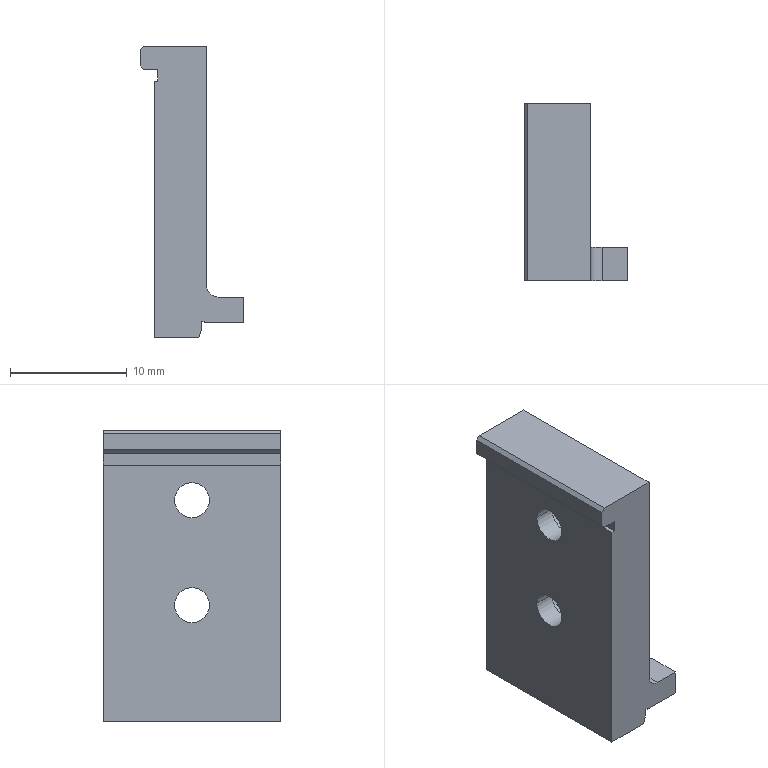Part | NX | 1 solid | 31 faces | box 8.9 x 15.2 x 25 mm | volume 1620 mm3 | plane 22 | cylinder 9 | commonest cylinder face diameters 3 x4 5 x4 2 x1
STEP:
#1=CARTESIAN_POINT('',(-1.77,0.,-1.43));
#2=VERTEX_POINT('',#1);
#3=CARTESIAN_POINT('',(-2.025,0.,-2.13));
#4=VERTEX_POINT('',#3);
#5=CARTESIAN_POINT('',(-1.25,0.,0.));
#6=DIRECTION('',(-0.342,0.,-0.9397));
#7=VECTOR('',#6,1000.);
#8=LINE('',#5,#7);
#9=EDGE_CURVE('',#2,#4,#8,.T.);
#10=ORIENTED_EDGE('',*,*,#9,.T.);
#11=CARTESIAN_POINT('',(-5.85,0.,-2.13));
#12=VERTEX_POINT('',#11);
#13=CARTESIAN_POINT('',(0.,0.,-2.13));
#14=DIRECTION('',(1.,0.,0.));
#15=VECTOR('',#14,1000.);
#16=LINE('',#13,#15);
#17=EDGE_CURVE('',#12,#4,#16,.T.);
#18=ORIENTED_EDGE('',*,*,#17,.F.);
#19=CARTESIAN_POINT('',(-5.85,0.,19.87));
#20=VERTEX_POINT('',#19);
#21=CARTESIAN_POINT('',(-5.85,0.,0.));
#22=DIRECTION('',(0.,0.,1.));
#23=VECTOR('',#22,1000.);
#24=LINE('',#21,#23);
#25=EDGE_CURVE('',#12,#20,#24,.T.);
#26=ORIENTED_EDGE('',*,*,#25,.T.);
#27=CARTESIAN_POINT('',(-5.55,0.,19.87));
#28=VERTEX_POINT('',#27);
#29=CARTESIAN_POINT('',(0.,0.,19.87));
#30=DIRECTION('',(1.,0.,0.));
#31=VECTOR('',#30,1000.);
#32=LINE('',#29,#31);
#33=EDGE_CURVE('',#20,#28,#32,.T.);
#34=ORIENTED_EDGE('',*,*,#33,.T.);
#35=CARTESIAN_POINT('',(-5.55,0.,20.87));
#36=VERTEX_POINT('',#35);
#37=CARTESIAN_POINT('',(-5.55,0.,0.));
#38=DIRECTION('',(0.,0.,1.));
#39=VECTOR('',#38,1000.);
#40=LINE('',#37,#39);
#41=EDGE_CURVE('',#28,#36,#40,.T.);
#42=ORIENTED_EDGE('',*,*,#41,.T.);
#43=CARTESIAN_POINT('',(-6.75,0.,20.87));
#44=VERTEX_POINT('',#43);
#45=CARTESIAN_POINT('',(0.,0.,20.87));
#46=DIRECTION('',(-1.,0.,0.));
#47=VECTOR('',#46,1000.);
#48=LINE('',#45,#47);
#49=EDGE_CURVE('',#36,#44,#48,.T.);
#50=ORIENTED_EDGE('',*,*,#49,.T.);
#51=CARTESIAN_POINT('',(-7.05,0.,21.17));
#52=VERTEX_POINT('',#51);
#53=CARTESIAN_POINT('',(14.12,0.,0.));
#54=DIRECTION('',(0.7071,0.,-0.7071));
#55=VECTOR('',#54,1000.);
#56=LINE('',#53,#55);
#57=EDGE_CURVE('',#52,#44,#56,.T.);
#58=ORIENTED_EDGE('',*,*,#57,.F.);
#59=CARTESIAN_POINT('',(-7.05,0.,22.57));
#60=VERTEX_POINT('',#59);
#61=CARTESIAN_POINT('',(-7.05,0.,0.));
#62=DIRECTION('',(0.,0.,1.));
#63=VECTOR('',#62,1000.);
#64=LINE('',#61,#63);
#65=EDGE_CURVE('',#52,#60,#64,.T.);
#66=ORIENTED_EDGE('',*,*,#65,.T.);
#67=CARTESIAN_POINT('',(-6.75,0.,22.87));
#68=VERTEX_POINT('',#67);
#69=CARTESIAN_POINT('',(-29.62,0.,0.));
#70=DIRECTION('',(0.7071,0.,0.7071));
#71=VECTOR('',#70,1000.);
#72=LINE('',#69,#71);
#73=EDGE_CURVE('',#60,#68,#72,.T.);
#74=ORIENTED_EDGE('',*,*,#73,.T.);
#75=CARTESIAN_POINT('',(-1.35,0.,22.87));
#76=VERTEX_POINT('',#75);
#77=CARTESIAN_POINT('',(0.,0.,22.87));
#78=DIRECTION('',(1.,0.,0.));
#79=VECTOR('',#78,1000.);
#80=LINE('',#77,#79);
#81=EDGE_CURVE('',#68,#76,#80,.T.);
#82=ORIENTED_EDGE('',*,*,#81,.T.);
#83=CARTESIAN_POINT('',(-1.35,0.,-0.83));
#84=VERTEX_POINT('',#83);
#85=CARTESIAN_POINT('',(-1.35,0.,0.));
#86=DIRECTION('',(0.,0.,-1.));
#87=VECTOR('',#86,1000.);
#88=LINE('',#85,#87);
#89=EDGE_CURVE('',#76,#84,#88,.T.);
#90=ORIENTED_EDGE('',*,*,#89,.T.);
#91=CARTESIAN_POINT('',(-1.57,0.,-0.83));
#92=VERTEX_POINT('',#91);
#93=CARTESIAN_POINT('',(0.,0.,-0.83));
#94=DIRECTION('',(1.,0.,0.));
#95=VECTOR('',#94,1000.);
#96=LINE('',#93,#95);
#97=EDGE_CURVE('',#92,#84,#96,.T.);
#98=ORIENTED_EDGE('',*,*,#97,.F.);
#99=CARTESIAN_POINT('',(-1.57,0.,-0.73));
#100=VERTEX_POINT('',#99);
#101=CARTESIAN_POINT('',(-1.57,0.,0.));
#102=DIRECTION('',(0.,0.,-1.));
#103=VECTOR('',#102,1000.);
#104=LINE('',#101,#103);
#105=EDGE_CURVE('',#100,#92,#104,.T.);
#106=ORIENTED_EDGE('',*,*,#105,.F.);
#107=CARTESIAN_POINT('',(-1.77,0.,-0.73));
#108=VERTEX_POINT('',#107);
#109=CARTESIAN_POINT('',(0.,0.,-0.73));
#110=DIRECTION('',(-1.,0.,0.));
#111=VECTOR('',#110,1000.);
#112=LINE('',#109,#111);
#113=EDGE_CURVE('',#100,#108,#112,.T.);
#114=ORIENTED_EDGE('',*,*,#113,.T.);
#115=CARTESIAN_POINT('',(-1.77,0.,0.));
#116=DIRECTION('',(0.,0.,-1.));
#117=VECTOR('',#116,1000.);
#118=LINE('',#115,#117);
#119=EDGE_CURVE('',#108,#2,#118,.T.);
#120=ORIENTED_EDGE('',*,*,#119,.T.);
#121=EDGE_LOOP('',(#10,#18,#26,#34,#42,#50,#58,#66,#74,#82,#90,#98,#106,#114,#120));
#122=FACE_BOUND('',#121,.T.);
#123=CARTESIAN_POINT('',(0.,0.,0.));
#124=DIRECTION('',(0.,-1.,0.));
#125=DIRECTION('',(0.,0.,-1.));
#126=AXIS2_PLACEMENT_3D('',#123,#124,#125);
#127=PLANE('',#126);
#128=ADVANCED_FACE('',(#122),#127,.F.);
#129=CARTESIAN_POINT('',(-1.77,-15.2,-1.43));
#130=VERTEX_POINT('',#129);
#131=CARTESIAN_POINT('',(-1.77,0.,-1.43));
#132=DIRECTION('',(0.,-1.,0.));
#133=VECTOR('',#132,1000.);
#134=LINE('',#131,#133);
#135=EDGE_CURVE('',#2,#130,#134,.T.);
#136=ORIENTED_EDGE('',*,*,#135,.F.);
#137=ORIENTED_EDGE('',*,*,#119,.F.);
#138=CARTESIAN_POINT('',(-1.77,-15.2,-0.73));
#139=VERTEX_POINT('',#138);
#140=CARTESIAN_POINT('',(-1.77,-15.2,-0.73));
#141=DIRECTION('',(0.,1.,0.));
#142=VECTOR('',#141,1000.);
#143=LINE('',#140,#142);
#144=EDGE_CURVE('',#139,#108,#143,.T.);
#145=ORIENTED_EDGE('',*,*,#144,.F.);
#146=CARTESIAN_POINT('',(-1.77,-15.2,0.));
#147=DIRECTION('',(0.,0.,1.));
#148=VECTOR('',#147,1000.);
#149=LINE('',#146,#148);
#150=EDGE_CURVE('',#130,#139,#149,.T.);
#151=ORIENTED_EDGE('',*,*,#150,.F.);
#152=EDGE_LOOP('',(#136,#137,#145,#151));
#153=FACE_BOUND('',#152,.T.);
#154=CARTESIAN_POINT('',(-1.77,0.,-0.93));
#155=DIRECTION('',(1.,0.,0.));
#156=DIRECTION('',(0.,1.,0.));
#157=AXIS2_PLACEMENT_3D('',#154,#155,#156);
#158=PLANE('',#157);
#159=ADVANCED_FACE('',(#153),#158,.T.);
#160=CARTESIAN_POINT('',(-0.35,-15.2,1.37));
#161=VERTEX_POINT('',#160);
#162=CARTESIAN_POINT('',(1.85,-15.2,1.37));
#163=VERTEX_POINT('',#162);
#164=CARTESIAN_POINT('',(0.,-15.2,1.37));
#165=DIRECTION('',(1.,0.,0.));
#166=VECTOR('',#165,1000.);
#167=LINE('',#164,#166);
#168=EDGE_CURVE('',#161,#163,#167,.T.);
#169=ORIENTED_EDGE('',*,*,#168,.F.);
#170=CARTESIAN_POINT('',(-1.35,-15.2,2.37));
#171=VERTEX_POINT('',#170);
#172=CARTESIAN_POINT('',(-0.35,-15.2,2.37));
#173=DIRECTION('',(0.,1.,0.));
#174=DIRECTION('',(-1.,0.,0.));
#175=AXIS2_PLACEMENT_3D('',#172,#173,#174);
#176=CIRCLE('',#175,1.);
#177=EDGE_CURVE('',#161,#171,#176,.T.);
#178=ORIENTED_EDGE('',*,*,#177,.T.);
#179=CARTESIAN_POINT('',(-1.35,-15.2,22.87));
#180=VERTEX_POINT('',#179);
#181=CARTESIAN_POINT('',(-1.35,-15.2,0.));
#182=DIRECTION('',(0.,0.,1.));
#183=VECTOR('',#182,1000.);
#184=LINE('',#181,#183);
#185=EDGE_CURVE('',#171,#180,#184,.T.);
#186=ORIENTED_EDGE('',*,*,#185,.T.);
#187=CARTESIAN_POINT('',(-6.75,-15.2,22.87));
#188=VERTEX_POINT('',#187);
#189=CARTESIAN_POINT('',(0.,-15.2,22.87));
#190=DIRECTION('',(-1.,0.,0.));
#191=VECTOR('',#190,1000.);
#192=LINE('',#189,#191);
#193=EDGE_CURVE('',#180,#188,#192,.T.);
#194=ORIENTED_EDGE('',*,*,#193,.T.);
#195=CARTESIAN_POINT('',(-7.05,-15.2,22.57));
#196=VERTEX_POINT('',#195);
#197=CARTESIAN_POINT('',(-29.62,-15.2,0.));
#198=DIRECTION('',(-0.7071,0.,-0.7071));
#199=VECTOR('',#198,1000.);
#200=LINE('',#197,#199);
#201=EDGE_CURVE('',#188,#196,#200,.T.);
#202=ORIENTED_EDGE('',*,*,#201,.T.);
#203=CARTESIAN_POINT('',(-7.05,-15.2,21.17));
#204=VERTEX_POINT('',#203);
#205=CARTESIAN_POINT('',(-7.05,-15.2,0.));
#206=DIRECTION('',(0.,0.,-1.));
#207=VECTOR('',#206,1000.);
#208=LINE('',#205,#207);
#209=EDGE_CURVE('',#196,#204,#208,.T.);
#210=ORIENTED_EDGE('',*,*,#209,.T.);
#211=CARTESIAN_POINT('',(-6.75,-15.2,20.87));
#212=VERTEX_POINT('',#211);
#213=CARTESIAN_POINT('',(14.12,-15.2,0.));
#214=DIRECTION('',(-0.7071,0.,0.7071));
#215=VECTOR('',#214,1000.);
#216=LINE('',#213,#215);
#217=EDGE_CURVE('',#212,#204,#216,.T.);
#218=ORIENTED_EDGE('',*,*,#217,.F.);
#219=CARTESIAN_POINT('',(-5.55,-15.2,20.87));
#220=VERTEX_POINT('',#219);
#221=CARTESIAN_POINT('',(0.,-15.2,20.87));
#222=DIRECTION('',(1.,0.,0.));
#223=VECTOR('',#222,1000.);
#224=LINE('',#221,#223);
#225=EDGE_CURVE('',#212,#220,#224,.T.);
#226=ORIENTED_EDGE('',*,*,#225,.T.);
#227=CARTESIAN_POINT('',(-5.55,-15.2,19.87));
#228=VERTEX_POINT('',#227);
#229=CARTESIAN_POINT('',(-5.55,-15.2,0.));
#230=DIRECTION('',(0.,0.,-1.));
#231=VECTOR('',#230,1000.);
#232=LINE('',#229,#231);
#233=EDGE_CURVE('',#220,#228,#232,.T.);
#234=ORIENTED_EDGE('',*,*,#233,.T.);
#235=CARTESIAN_POINT('',(-5.85,-15.2,19.87));
#236=VERTEX_POINT('',#235);
#237=CARTESIAN_POINT('',(0.,-15.2,19.87));
#238=DIRECTION('',(-1.,0.,0.));
#239=VECTOR('',#238,1000.);
#240=LINE('',#237,#239);
#241=EDGE_CURVE('',#228,#236,#240,.T.);
#242=ORIENTED_EDGE('',*,*,#241,.T.);
#243=CARTESIAN_POINT('',(-5.85,-15.2,-2.13));
#244=VERTEX_POINT('',#243);
#245=CARTESIAN_POINT('',(-5.85,-15.2,0.));
#246=DIRECTION('',(0.,0.,-1.));
#247=VECTOR('',#246,1000.);
#248=LINE('',#245,#247);
#249=EDGE_CURVE('',#236,#244,#248,.T.);
#250=ORIENTED_EDGE('',*,*,#249,.T.);
#251=CARTESIAN_POINT('',(-2.025,-15.2,-2.13));
#252=VERTEX_POINT('',#251);
#253=CARTESIAN_POINT('',(0.,-15.2,-2.13));
#254=DIRECTION('',(-1.,0.,0.));
#255=VECTOR('',#254,1000.);
#256=LINE('',#253,#255);
#257=EDGE_CURVE('',#252,#244,#256,.T.);
#258=ORIENTED_EDGE('',*,*,#257,.F.);
#259=CARTESIAN_POINT('',(-1.25,-15.2,0.));
#260=DIRECTION('',(0.342,0.,0.9397));
#261=VECTOR('',#260,1000.);
#262=LINE('',#259,#261);
#263=EDGE_CURVE('',#252,#130,#262,.T.);
#264=ORIENTED_EDGE('',*,*,#263,.T.);
#265=ORIENTED_EDGE('',*,*,#150,.T.);
#266=CARTESIAN_POINT('',(-1.57,-15.2,-0.73));
#267=VERTEX_POINT('',#266);
#268=CARTESIAN_POINT('',(0.,-15.2,-0.73));
#269=DIRECTION('',(1.,0.,0.));
#270=VECTOR('',#269,1000.);
#271=LINE('',#268,#270);
#272=EDGE_CURVE('',#139,#267,#271,.T.);
#273=ORIENTED_EDGE('',*,*,#272,.T.);
#274=CARTESIAN_POINT('',(-1.57,-15.2,-0.83));
#275=VERTEX_POINT('',#274);
#276=CARTESIAN_POINT('',(-1.57,-15.2,0.));
#277=DIRECTION('',(0.,0.,1.));
#278=VECTOR('',#277,1000.);
#279=LINE('',#276,#278);
#280=EDGE_CURVE('',#275,#267,#279,.T.);
#281=ORIENTED_EDGE('',*,*,#280,.F.);
#282=CARTESIAN_POINT('',(1.85,-15.2,-0.83));
#283=VERTEX_POINT('',#282);
#284=CARTESIAN_POINT('',(0.,-15.2,-0.83));
#285=DIRECTION('',(1.,0.,0.));
#286=VECTOR('',#285,1000.);
#287=LINE('',#284,#286);
#288=EDGE_CURVE('',#275,#283,#287,.T.);
#289=ORIENTED_EDGE('',*,*,#288,.T.);
#290=CARTESIAN_POINT('',(1.85,-15.2,0.));
#291=DIRECTION('',(0.,0.,1.));
#292=VECTOR('',#291,1000.);
#293=LINE('',#290,#292);
#294=EDGE_CURVE('',#283,#163,#293,.T.);
#295=ORIENTED_EDGE('',*,*,#294,.T.);
#296=EDGE_LOOP('',(#169,#178,#186,#194,#202,#210,#218,#226,#234,#242,#250,#258,#264,#265,#273,#281,#289,#295));
#297=FACE_BOUND('',#296,.T.);
#298=CARTESIAN_POINT('',(-1.35,-15.2,0.));
#299=DIRECTION('',(0.,1.,0.));
#300=DIRECTION('',(1.,0.,0.));
#301=AXIS2_PLACEMENT_3D('',#298,#299,#300);
#302=PLANE('',#301);
#303=ADVANCED_FACE('',(#297),#302,.F.);
#304=CARTESIAN_POINT('',(-4.05,-5.1,7.87));
#305=VERTEX_POINT('',#304);
#306=CARTESIAN_POINT('',(-4.05,-10.1,7.87));
#307=VERTEX_POINT('',#306);
#308=CARTESIAN_POINT('',(-4.05,-7.6,7.87));
#309=DIRECTION('',(1.,0.,0.));
#310=DIRECTION('',(0.,-1.,0.));
#311=AXIS2_PLACEMENT_3D('',#308,#309,#310);
#312=CIRCLE('',#311,2.5);
#313=EDGE_CURVE('',#305,#307,#312,.T.);
#314=ORIENTED_EDGE('',*,*,#313,.T.);
#315=CARTESIAN_POINT('',(-4.05,-7.6,7.87));
#316=DIRECTION('',(1.,0.,0.));
#317=DIRECTION('',(0.,-1.,0.));
#318=AXIS2_PLACEMENT_3D('',#315,#316,#317);
#319=CIRCLE('',#318,2.5);
#320=EDGE_CURVE('',#307,#305,#319,.T.);
#321=ORIENTED_EDGE('',*,*,#320,.T.);
#322=EDGE_LOOP('',(#314,#321));
#323=FACE_BOUND('',#322,.T.);
#324=CARTESIAN_POINT('',(-4.05,-6.1,7.87));
#325=VERTEX_POINT('',#324);
#326=CARTESIAN_POINT('',(-4.05,-9.1,7.87));
#327=VERTEX_POINT('',#326);
#328=CARTESIAN_POINT('',(-4.05,-7.6,7.87));
#329=DIRECTION('',(1.,0.,0.));
#330=DIRECTION('',(0.,-1.,0.));
#331=AXIS2_PLACEMENT_3D('',#328,#329,#330);
#332=CIRCLE('',#331,1.5);
#333=EDGE_CURVE('',#325,#327,#332,.T.);
#334=ORIENTED_EDGE('',*,*,#333,.F.);
#335=CARTESIAN_POINT('',(-4.05,-7.6,7.87));
#336=DIRECTION('',(1.,0.,0.));
#337=DIRECTION('',(0.,-1.,0.));
#338=AXIS2_PLACEMENT_3D('',#335,#336,#337);
#339=CIRCLE('',#338,1.5);
#340=EDGE_CURVE('',#327,#325,#339,.T.);
#341=ORIENTED_EDGE('',*,*,#340,.F.);
#342=EDGE_LOOP('',(#334,#341));
#343=FACE_BOUND('',#342,.T.);
#344=CARTESIAN_POINT('',(-4.05,-7.6,7.87));
#345=DIRECTION('',(-1.,0.,0.));
#346=DIRECTION('',(0.,0.,1.));
#347=AXIS2_PLACEMENT_3D('',#344,#345,#346);
#348=PLANE('',#347);
#349=ADVANCED_FACE('',(#323,#343),#348,.F.);
#350=ORIENTED_EDGE('',*,*,#257,.T.);
#351=CARTESIAN_POINT('',(-5.85,0.,-2.13));
#352=DIRECTION('',(0.,1.,0.));
#353=VECTOR('',#352,1000.);
#354=LINE('',#351,#353);
#355=EDGE_CURVE('',#244,#12,#354,.T.);
#356=ORIENTED_EDGE('',*,*,#355,.T.);
#357=ORIENTED_EDGE('',*,*,#17,.T.);
#358=CARTESIAN_POINT('',(-2.025,0.,-2.13));
#359=DIRECTION('',(0.,-1.,0.));
#360=VECTOR('',#359,1000.);
#361=LINE('',#358,#360);
#362=EDGE_CURVE('',#4,#252,#361,.T.);
#363=ORIENTED_EDGE('',*,*,#362,.T.);
#364=EDGE_LOOP('',(#350,#356,#357,#363));
#365=FACE_BOUND('',#364,.T.);
#366=CARTESIAN_POINT('',(0.,0.,-2.13));
#367=DIRECTION('',(0.,0.,1.));
#368=DIRECTION('',(1.,0.,0.));
#369=AXIS2_PLACEMENT_3D('',#366,#367,#368);
#370=PLANE('',#369);
#371=ADVANCED_FACE('',(#365),#370,.F.);
#372=ORIENTED_EDGE('',*,*,#9,.F.);
#373=ORIENTED_EDGE('',*,*,#135,.T.);
#374=ORIENTED_EDGE('',*,*,#263,.F.);
#375=ORIENTED_EDGE('',*,*,#362,.F.);
#376=EDGE_LOOP('',(#372,#373,#374,#375));
#377=FACE_BOUND('',#376,.T.);
#378=CARTESIAN_POINT('',(-2.025,-15.2,-2.13));
#379=DIRECTION('',(0.9397,0.,-0.342));
#380=DIRECTION('',(0.,-1.,0.));
#381=AXIS2_PLACEMENT_3D('',#378,#379,#380);
#382=PLANE('',#381);
#383=ADVANCED_FACE('',(#377),#382,.T.);
#384=CARTESIAN_POINT('',(-5.85,0.,19.87));
#385=DIRECTION('',(0.,-1.,0.));
#386=VECTOR('',#385,1000.);
#387=LINE('',#384,#386);
#388=EDGE_CURVE('',#20,#236,#387,.T.);
#389=ORIENTED_EDGE('',*,*,#388,.T.);
#390=ORIENTED_EDGE('',*,*,#241,.F.);
#391=CARTESIAN_POINT('',(-5.55,0.,19.87));
#392=DIRECTION('',(0.,-1.,0.));
#393=VECTOR('',#392,1000.);
#394=LINE('',#391,#393);
#395=EDGE_CURVE('',#28,#228,#394,.T.);
#396=ORIENTED_EDGE('',*,*,#395,.F.);
#397=ORIENTED_EDGE('',*,*,#33,.F.);
#398=EDGE_LOOP('',(#389,#390,#396,#397));
#399=FACE_BOUND('',#398,.T.);
#400=CARTESIAN_POINT('',(-4.85,0.,19.87));
#401=DIRECTION('',(0.,0.,1.));
#402=DIRECTION('',(1.,0.,0.));
#403=AXIS2_PLACEMENT_3D('',#400,#401,#402);
#404=PLANE('',#403);
#405=ADVANCED_FACE('',(#399),#404,.T.);
#406=ORIENTED_EDGE('',*,*,#395,.T.);
#407=ORIENTED_EDGE('',*,*,#233,.F.);
#408=CARTESIAN_POINT('',(-5.55,0.,20.87));
#409=DIRECTION('',(0.,-1.,0.));
#410=VECTOR('',#409,1000.);
#411=LINE('',#408,#410);
#412=EDGE_CURVE('',#36,#220,#411,.T.);
#413=ORIENTED_EDGE('',*,*,#412,.F.);
#414=ORIENTED_EDGE('',*,*,#41,.F.);
#415=EDGE_LOOP('',(#406,#407,#413,#414));
#416=FACE_BOUND('',#415,.T.);
#417=CARTESIAN_POINT('',(-5.55,0.,19.87));
#418=DIRECTION('',(-1.,0.,0.));
#419=DIRECTION('',(0.,0.,1.));
#420=AXIS2_PLACEMENT_3D('',#417,#418,#419);
#421=PLANE('',#420);
#422=ADVANCED_FACE('',(#416),#421,.T.);
#423=CARTESIAN_POINT('',(-6.75,0.,20.87));
#424=DIRECTION('',(0.,1.,0.));
#425=VECTOR('',#424,1000.);
#426=LINE('',#423,#425);
#427=EDGE_CURVE('',#212,#44,#426,.T.);
#428=ORIENTED_EDGE('',*,*,#427,.T.);
#429=ORIENTED_EDGE('',*,*,#49,.F.);
#430=ORIENTED_EDGE('',*,*,#412,.T.);
#431=ORIENTED_EDGE('',*,*,#225,.F.);
#432=EDGE_LOOP('',(#428,#429,#430,#431));
#433=FACE_BOUND('',#432,.T.);
#434=CARTESIAN_POINT('',(-4.85,0.,20.87));
#435=DIRECTION('',(0.,0.,-1.));
#436=DIRECTION('',(0.,-1.,0.));
#437=AXIS2_PLACEMENT_3D('',#434,#435,#436);
#438=PLANE('',#437);
#439=ADVANCED_FACE('',(#433),#438,.T.);
#440=CARTESIAN_POINT('',(-7.05,0.,22.57));
#441=DIRECTION('',(0.,-1.,0.));
#442=VECTOR('',#441,1000.);
#443=LINE('',#440,#442);
#444=EDGE_CURVE('',#60,#196,#443,.T.);
#445=ORIENTED_EDGE('',*,*,#444,.F.);
#446=ORIENTED_EDGE('',*,*,#65,.F.);
#447=CARTESIAN_POINT('',(-7.05,0.,21.17));
#448=DIRECTION('',(0.,-1.,0.));
#449=VECTOR('',#448,1000.);
#450=LINE('',#447,#449);
#451=EDGE_CURVE('',#52,#204,#450,.T.);
#452=ORIENTED_EDGE('',*,*,#451,.T.);
#453=ORIENTED_EDGE('',*,*,#209,.F.);
#454=EDGE_LOOP('',(#445,#446,#452,#453));
#455=FACE_BOUND('',#454,.T.);
#456=CARTESIAN_POINT('',(-7.05,0.,20.87));
#457=DIRECTION('',(-1.,0.,0.));
#458=DIRECTION('',(0.,0.,1.));
#459=AXIS2_PLACEMENT_3D('',#456,#457,#458);
#460=PLANE('',#459);
#461=ADVANCED_FACE('',(#455),#460,.T.);
#462=CARTESIAN_POINT('',(-6.75,0.,22.87));
#463=DIRECTION('',(0.,1.,0.));
#464=VECTOR('',#463,1000.);
#465=LINE('',#462,#464);
#466=EDGE_CURVE('',#188,#68,#465,.T.);
#467=ORIENTED_EDGE('',*,*,#466,.F.);
#468=ORIENTED_EDGE('',*,*,#193,.F.);
#469=CARTESIAN_POINT('',(-1.35,0.,22.87));
#470=DIRECTION('',(0.,-1.,0.));
#471=VECTOR('',#470,1000.);
#472=LINE('',#469,#471);
#473=EDGE_CURVE('',#76,#180,#472,.T.);
#474=ORIENTED_EDGE('',*,*,#473,.F.);
#475=ORIENTED_EDGE('',*,*,#81,.F.);
#476=EDGE_LOOP('',(#467,#468,#474,#475));
#477=FACE_BOUND('',#476,.T.);
#478=CARTESIAN_POINT('',(-6.05,0.,22.87));
#479=DIRECTION('',(0.,0.,1.));
#480=DIRECTION('',(1.,0.,0.));
#481=AXIS2_PLACEMENT_3D('',#478,#479,#480);
#482=PLANE('',#481);
#483=ADVANCED_FACE('',(#477),#482,.T.);
#484=ORIENTED_EDGE('',*,*,#185,.F.);
#485=CARTESIAN_POINT('',(-1.35,-12.3,2.37));
#486=VERTEX_POINT('',#485);
#487=CARTESIAN_POINT('',(-1.35,-15.285,2.37));
#488=DIRECTION('',(0.,1.,0.));
#489=VECTOR('',#488,1000.);
#490=LINE('',#487,#489);
#491=EDGE_CURVE('',#171,#486,#490,.T.);
#492=ORIENTED_EDGE('',*,*,#491,.T.);
#493=CARTESIAN_POINT('',(-1.35,-12.3,-0.83));
#494=VERTEX_POINT('',#493);
#495=CARTESIAN_POINT('',(-1.35,-12.3,0.));
#496=DIRECTION('',(0.,0.,-1.));
#497=VECTOR('',#496,1000.);
#498=LINE('',#495,#497);
#499=EDGE_CURVE('',#486,#494,#498,.T.);
#500=ORIENTED_EDGE('',*,*,#499,.T.);
#501=CARTESIAN_POINT('',(-1.35,0.,-0.83));
#502=DIRECTION('',(0.,1.,0.));
#503=VECTOR('',#502,1000.);
#504=LINE('',#501,#503);
#505=EDGE_CURVE('',#494,#84,#504,.T.);
#506=ORIENTED_EDGE('',*,*,#505,.T.);
#507=ORIENTED_EDGE('',*,*,#89,.F.);
#508=ORIENTED_EDGE('',*,*,#473,.T.);
#509=EDGE_LOOP('',(#484,#492,#500,#506,#507,#508));
#510=FACE_BOUND('',#509,.T.);
#511=CARTESIAN_POINT('',(-1.35,-10.1,16.87));
#512=VERTEX_POINT('',#511);
#513=CARTESIAN_POINT('',(-1.35,-5.1,16.87));
#514=VERTEX_POINT('',#513);
#515=CARTESIAN_POINT('',(-1.35,-7.6,16.87));
#516=DIRECTION('',(1.,0.,0.));
#517=DIRECTION('',(0.,-1.,0.));
#518=AXIS2_PLACEMENT_3D('',#515,#516,#517);
#519=CIRCLE('',#518,2.5);
#520=EDGE_CURVE('',#512,#514,#519,.T.);
#521=ORIENTED_EDGE('',*,*,#520,.F.);
#522=CARTESIAN_POINT('',(-1.35,-7.6,16.87));
#523=DIRECTION('',(1.,0.,0.));
#524=DIRECTION('',(0.,-1.,0.));
#525=AXIS2_PLACEMENT_3D('',#522,#523,#524);
#526=CIRCLE('',#525,2.5);
#527=EDGE_CURVE('',#514,#512,#526,.T.);
#528=ORIENTED_EDGE('',*,*,#527,.F.);
#529=EDGE_LOOP('',(#521,#528));
#530=FACE_BOUND('',#529,.T.);
#531=CARTESIAN_POINT('',(-1.35,-10.1,7.87));
#532=VERTEX_POINT('',#531);
#533=CARTESIAN_POINT('',(-1.35,-5.1,7.87));
#534=VERTEX_POINT('',#533);
#535=CARTESIAN_POINT('',(-1.35,-7.6,7.87));
#536=DIRECTION('',(1.,0.,0.));
#537=DIRECTION('',(0.,-1.,0.));
#538=AXIS2_PLACEMENT_3D('',#535,#536,#537);
#539=CIRCLE('',#538,2.5);
#540=EDGE_CURVE('',#532,#534,#539,.T.);
#541=ORIENTED_EDGE('',*,*,#540,.F.);
#542=CARTESIAN_POINT('',(-1.35,-7.6,7.87));
#543=DIRECTION('',(1.,0.,0.));
#544=DIRECTION('',(0.,-1.,0.));
#545=AXIS2_PLACEMENT_3D('',#542,#543,#544);
#546=CIRCLE('',#545,2.5);
#547=EDGE_CURVE('',#534,#532,#546,.T.);
#548=ORIENTED_EDGE('',*,*,#547,.F.);
#549=EDGE_LOOP('',(#541,#548));
#550=FACE_BOUND('',#549,.T.);
#551=CARTESIAN_POINT('',(-1.35,0.,-1.13));
#552=DIRECTION('',(-1.,0.,0.));
#553=DIRECTION('',(0.,0.,1.));
#554=AXIS2_PLACEMENT_3D('',#551,#552,#553);
#555=PLANE('',#554);
#556=ADVANCED_FACE('',(#510,#530,#550),#555,.F.);
#557=ORIENTED_EDGE('',*,*,#491,.F.);
#558=ORIENTED_EDGE('',*,*,#177,.F.);
#559=CARTESIAN_POINT('',(-0.35,-12.3,1.37));
#560=VERTEX_POINT('',#559);
#561=CARTESIAN_POINT('',(-0.35,-15.2,1.37));
#562=DIRECTION('',(0.,1.,0.));
#563=VECTOR('',#562,1000.);
#564=LINE('',#561,#563);
#565=EDGE_CURVE('',#161,#560,#564,.T.);
#566=ORIENTED_EDGE('',*,*,#565,.T.);
#567=CARTESIAN_POINT('',(-0.35,-12.3,2.37));
#568=DIRECTION('',(0.,1.,0.));
#569=DIRECTION('',(-1.,0.,0.));
#570=AXIS2_PLACEMENT_3D('',#567,#568,#569);
#571=CIRCLE('',#570,1.);
#572=EDGE_CURVE('',#560,#486,#571,.T.);
#573=ORIENTED_EDGE('',*,*,#572,.T.);
#574=EDGE_LOOP('',(#557,#558,#566,#573));
#575=FACE_BOUND('',#574,.T.);
#576=CARTESIAN_POINT('',(-0.35,-15.285,2.37));
#577=DIRECTION('',(0.,1.,0.));
#578=DIRECTION('',(-1.,0.,0.));
#579=AXIS2_PLACEMENT_3D('',#576,#577,#578);
#580=CYLINDRICAL_SURFACE('',#579,1.);
#581=ADVANCED_FACE('',(#575),#580,.F.);
#582=CARTESIAN_POINT('',(1.85,-12.3,1.37));
#583=VERTEX_POINT('',#582);
#584=CARTESIAN_POINT('',(1.85,-12.3,-0.83));
#585=VERTEX_POINT('',#584);
#586=CARTESIAN_POINT('',(1.85,-12.3,0.));
#587=DIRECTION('',(0.,0.,-1.));
#588=VECTOR('',#587,1000.);
#589=LINE('',#586,#588);
#590=EDGE_CURVE('',#583,#585,#589,.T.);
#591=ORIENTED_EDGE('',*,*,#590,.T.);
#592=CARTESIAN_POINT('',(0.,-12.3,-0.83));
#593=DIRECTION('',(1.,0.,0.));
#594=VECTOR('',#593,1000.);
#595=LINE('',#592,#594);
#596=EDGE_CURVE('',#494,#585,#595,.T.);
#597=ORIENTED_EDGE('',*,*,#596,.F.);
#598=ORIENTED_EDGE('',*,*,#499,.F.);
#599=ORIENTED_EDGE('',*,*,#572,.F.);
#600=CARTESIAN_POINT('',(0.,-12.3,1.37));
#601=DIRECTION('',(-1.,0.,0.));
#602=VECTOR('',#601,1000.);
#603=LINE('',#600,#602);
#604=EDGE_CURVE('',#583,#560,#603,.T.);
#605=ORIENTED_EDGE('',*,*,#604,.F.);
#606=EDGE_LOOP('',(#591,#597,#598,#599,#605));
#607=FACE_BOUND('',#606,.T.);
#608=CARTESIAN_POINT('',(-1.77,-12.3,-0.83));
#609=DIRECTION('',(0.,-1.,0.));
#610=DIRECTION('',(0.,0.,-1.));
#611=AXIS2_PLACEMENT_3D('',#608,#609,#610);
#612=PLANE('',#611);
#613=ADVANCED_FACE('',(#607),#612,.F.);
#614=ORIENTED_EDGE('',*,*,#294,.F.);
#615=CARTESIAN_POINT('',(1.85,0.,-0.83));
#616=DIRECTION('',(0.,1.,0.));
#617=VECTOR('',#616,1000.);
#618=LINE('',#615,#617);
#619=EDGE_CURVE('',#283,#585,#618,.T.);
#620=ORIENTED_EDGE('',*,*,#619,.T.);
#621=ORIENTED_EDGE('',*,*,#590,.F.);
#622=CARTESIAN_POINT('',(1.85,0.,1.37));
#623=DIRECTION('',(0.,1.,0.));
#624=VECTOR('',#623,1000.);
#625=LINE('',#622,#624);
#626=EDGE_CURVE('',#163,#583,#625,.T.);
#627=ORIENTED_EDGE('',*,*,#626,.F.);
#628=EDGE_LOOP('',(#614,#620,#621,#627));
#629=FACE_BOUND('',#628,.T.);
#630=CARTESIAN_POINT('',(1.85,0.,52.77));
#631=DIRECTION('',(-1.,0.,0.));
#632=DIRECTION('',(0.,0.,1.));
#633=AXIS2_PLACEMENT_3D('',#630,#631,#632);
#634=PLANE('',#633);
#635=ADVANCED_FACE('',(#629),#634,.F.);
#636=ORIENTED_EDGE('',*,*,#313,.F.);
#637=CARTESIAN_POINT('',(-7.072,-5.1,7.87));
#638=DIRECTION('',(1.,0.,0.));
#639=VECTOR('',#638,1000.);
#640=LINE('',#637,#639);
#641=EDGE_CURVE('',#305,#534,#640,.T.);
#642=ORIENTED_EDGE('',*,*,#641,.T.);
#643=ORIENTED_EDGE('',*,*,#547,.T.);
#644=CARTESIAN_POINT('',(-7.072,-10.1,7.87));
#645=DIRECTION('',(1.,0.,0.));
#646=VECTOR('',#645,1000.);
#647=LINE('',#644,#646);
#648=EDGE_CURVE('',#307,#532,#647,.T.);
#649=ORIENTED_EDGE('',*,*,#648,.F.);
#650=EDGE_LOOP('',(#636,#642,#643,#649));
#651=FACE_BOUND('',#650,.T.);
#652=CARTESIAN_POINT('',(-7.072,-7.6,7.87));
#653=DIRECTION('',(1.,0.,0.));
#654=DIRECTION('',(0.,-1.,0.));
#655=AXIS2_PLACEMENT_3D('',#652,#653,#654);
#656=CYLINDRICAL_SURFACE('',#655,2.5);
#657=ADVANCED_FACE('',(#651),#656,.F.);
#658=ORIENTED_EDGE('',*,*,#604,.T.);
#659=ORIENTED_EDGE('',*,*,#565,.F.);
#660=ORIENTED_EDGE('',*,*,#168,.T.);
#661=ORIENTED_EDGE('',*,*,#626,.T.);
#662=EDGE_LOOP('',(#658,#659,#660,#661));
#663=FACE_BOUND('',#662,.T.);
#664=CARTESIAN_POINT('',(-1.35,-15.2,1.37));
#665=DIRECTION('',(0.,0.,-1.));
#666=DIRECTION('',(0.,-1.,0.));
#667=AXIS2_PLACEMENT_3D('',#664,#665,#666);
#668=PLANE('',#667);
#669=ADVANCED_FACE('',(#663),#668,.F.);
#670=ORIENTED_EDGE('',*,*,#97,.T.);
#671=ORIENTED_EDGE('',*,*,#505,.F.);
#672=ORIENTED_EDGE('',*,*,#596,.T.);
#673=ORIENTED_EDGE('',*,*,#619,.F.);
#674=ORIENTED_EDGE('',*,*,#288,.F.);
#675=CARTESIAN_POINT('',(-1.57,0.,-0.83));
#676=DIRECTION('',(0.,1.,0.));
#677=VECTOR('',#676,1000.);
#678=LINE('',#675,#677);
#679=EDGE_CURVE('',#275,#92,#678,.T.);
#680=ORIENTED_EDGE('',*,*,#679,.T.);
#681=EDGE_LOOP('',(#670,#671,#672,#673,#674,#680));
#682=FACE_BOUND('',#681,.T.);
#683=CARTESIAN_POINT('',(1.45,0.,-0.83));
#684=DIRECTION('',(0.,0.,-1.));
#685=DIRECTION('',(0.,-1.,0.));
#686=AXIS2_PLACEMENT_3D('',#683,#684,#685);
#687=PLANE('',#686);
#688=ADVANCED_FACE('',(#682),#687,.T.);
#689=CARTESIAN_POINT('',(-1.57,0.,-0.73));
#690=DIRECTION('',(0.,1.,0.));
#691=VECTOR('',#690,1000.);
#692=LINE('',#689,#691);
#693=EDGE_CURVE('',#267,#100,#692,.T.);
#694=ORIENTED_EDGE('',*,*,#693,.T.);
#695=ORIENTED_EDGE('',*,*,#105,.T.);
#696=ORIENTED_EDGE('',*,*,#679,.F.);
#697=ORIENTED_EDGE('',*,*,#280,.T.);
#698=EDGE_LOOP('',(#694,#695,#696,#697));
#699=FACE_BOUND('',#698,.T.);
#700=CARTESIAN_POINT('',(-1.57,1.52,-0.93));
#701=DIRECTION('',(-1.,0.,0.));
#702=DIRECTION('',(0.,0.,1.));
#703=AXIS2_PLACEMENT_3D('',#700,#701,#702);
#704=PLANE('',#703);
#705=ADVANCED_FACE('',(#699),#704,.T.);
#706=ORIENTED_EDGE('',*,*,#144,.T.);
#707=ORIENTED_EDGE('',*,*,#113,.F.);
#708=ORIENTED_EDGE('',*,*,#693,.F.);
#709=ORIENTED_EDGE('',*,*,#272,.F.);
#710=EDGE_LOOP('',(#706,#707,#708,#709));
#711=FACE_BOUND('',#710,.T.);
#712=CARTESIAN_POINT('',(-1.57,1.52,-0.73));
#713=DIRECTION('',(0.,0.,-1.));
#714=DIRECTION('',(0.,-1.,0.));
#715=AXIS2_PLACEMENT_3D('',#712,#713,#714);
#716=PLANE('',#715);
#717=ADVANCED_FACE('',(#711),#716,.T.);
#718=CARTESIAN_POINT('',(-4.05,-5.1,16.87));
#719=VERTEX_POINT('',#718);
#720=CARTESIAN_POINT('',(-4.05,-10.1,16.87));
#721=VERTEX_POINT('',#720);
#722=CARTESIAN_POINT('',(-4.05,-7.6,16.87));
#723=DIRECTION('',(1.,0.,0.));
#724=DIRECTION('',(0.,-1.,0.));
#725=AXIS2_PLACEMENT_3D('',#722,#723,#724);
#726=CIRCLE('',#725,2.5);
#727=EDGE_CURVE('',#719,#721,#726,.T.);
#728=ORIENTED_EDGE('',*,*,#727,.F.);
#729=CARTESIAN_POINT('',(-7.072,-5.1,16.87));
#730=DIRECTION('',(1.,0.,0.));
#731=VECTOR('',#730,1000.);
#732=LINE('',#729,#731);
#733=EDGE_CURVE('',#719,#514,#732,.T.);
#734=ORIENTED_EDGE('',*,*,#733,.T.);
#735=ORIENTED_EDGE('',*,*,#527,.T.);
#736=CARTESIAN_POINT('',(-7.072,-10.1,16.87));
#737=DIRECTION('',(1.,0.,0.));
#738=VECTOR('',#737,1000.);
#739=LINE('',#736,#738);
#740=EDGE_CURVE('',#721,#512,#739,.T.);
#741=ORIENTED_EDGE('',*,*,#740,.F.);
#742=EDGE_LOOP('',(#728,#734,#735,#741));
#743=FACE_BOUND('',#742,.T.);
#744=CARTESIAN_POINT('',(-7.072,-7.6,16.87));
#745=DIRECTION('',(1.,0.,0.));
#746=DIRECTION('',(0.,-1.,0.));
#747=AXIS2_PLACEMENT_3D('',#744,#745,#746);
#748=CYLINDRICAL_SURFACE('',#747,2.5);
#749=ADVANCED_FACE('',(#743),#748,.F.);
#750=ORIENTED_EDGE('',*,*,#355,.F.);
#751=ORIENTED_EDGE('',*,*,#249,.F.);
#752=ORIENTED_EDGE('',*,*,#388,.F.);
#753=ORIENTED_EDGE('',*,*,#25,.F.);
#754=EDGE_LOOP('',(#750,#751,#752,#753));
#755=FACE_BOUND('',#754,.T.);
#756=CARTESIAN_POINT('',(-5.85,-9.1,16.87));
#757=VERTEX_POINT('',#756);
#758=CARTESIAN_POINT('',(-5.85,-6.1,16.87));
#759=VERTEX_POINT('',#758);
#760=CARTESIAN_POINT('',(-5.85,-7.6,16.87));
#761=DIRECTION('',(1.,0.,0.));
#762=DIRECTION('',(0.,-1.,0.));
#763=AXIS2_PLACEMENT_3D('',#760,#761,#762);
#764=CIRCLE('',#763,1.5);
#765=EDGE_CURVE('',#757,#759,#764,.T.);
#766=ORIENTED_EDGE('',*,*,#765,.T.);
#767=CARTESIAN_POINT('',(-5.85,-7.6,16.87));
#768=DIRECTION('',(1.,0.,0.));
#769=DIRECTION('',(0.,-1.,0.));
#770=AXIS2_PLACEMENT_3D('',#767,#768,#769);
#771=CIRCLE('',#770,1.5);
#772=EDGE_CURVE('',#759,#757,#771,.T.);
#773=ORIENTED_EDGE('',*,*,#772,.T.);
#774=EDGE_LOOP('',(#766,#773));
#775=FACE_BOUND('',#774,.T.);
#776=CARTESIAN_POINT('',(-5.85,-6.1,7.87));
#777=VERTEX_POINT('',#776);
#778=CARTESIAN_POINT('',(-5.85,-9.1,7.87));
#779=VERTEX_POINT('',#778);
#780=CARTESIAN_POINT('',(-5.85,-7.6,7.87));
#781=DIRECTION('',(1.,0.,0.));
#782=DIRECTION('',(0.,-1.,0.));
#783=AXIS2_PLACEMENT_3D('',#780,#781,#782);
#784=CIRCLE('',#783,1.5);
#785=EDGE_CURVE('',#777,#779,#784,.T.);
#786=ORIENTED_EDGE('',*,*,#785,.T.);
#787=CARTESIAN_POINT('',(-5.85,-7.6,7.87));
#788=DIRECTION('',(1.,0.,0.));
#789=DIRECTION('',(0.,-1.,0.));
#790=AXIS2_PLACEMENT_3D('',#787,#788,#789);
#791=CIRCLE('',#790,1.5);
#792=EDGE_CURVE('',#779,#777,#791,.T.);
#793=ORIENTED_EDGE('',*,*,#792,.T.);
#794=EDGE_LOOP('',(#786,#793));
#795=FACE_BOUND('',#794,.T.);
#796=CARTESIAN_POINT('',(-5.85,0.,-1.13));
#797=DIRECTION('',(-1.,0.,0.));
#798=DIRECTION('',(0.,0.,1.));
#799=AXIS2_PLACEMENT_3D('',#796,#797,#798);
#800=PLANE('',#799);
#801=ADVANCED_FACE('',(#755,#775,#795),#800,.T.);
#802=ORIENTED_EDGE('',*,*,#727,.T.);
#803=CARTESIAN_POINT('',(-4.05,-7.6,16.87));
#804=DIRECTION('',(1.,0.,0.));
#805=DIRECTION('',(0.,-1.,0.));
#806=AXIS2_PLACEMENT_3D('',#803,#804,#805);
#807=CIRCLE('',#806,2.5);
#808=EDGE_CURVE('',#721,#719,#807,.T.);
#809=ORIENTED_EDGE('',*,*,#808,.T.);
#810=EDGE_LOOP('',(#802,#809));
#811=FACE_BOUND('',#810,.T.);
#812=CARTESIAN_POINT('',(-4.05,-6.1,16.87));
#813=VERTEX_POINT('',#812);
#814=CARTESIAN_POINT('',(-4.05,-9.1,16.87));
#815=VERTEX_POINT('',#814);
#816=CARTESIAN_POINT('',(-4.05,-7.6,16.87));
#817=DIRECTION('',(1.,0.,0.));
#818=DIRECTION('',(0.,-1.,0.));
#819=AXIS2_PLACEMENT_3D('',#816,#817,#818);
#820=CIRCLE('',#819,1.5);
#821=EDGE_CURVE('',#813,#815,#820,.T.);
#822=ORIENTED_EDGE('',*,*,#821,.F.);
#823=CARTESIAN_POINT('',(-4.05,-7.6,16.87));
#824=DIRECTION('',(1.,0.,0.));
#825=DIRECTION('',(0.,-1.,0.));
#826=AXIS2_PLACEMENT_3D('',#823,#824,#825);
#827=CIRCLE('',#826,1.5);
#828=EDGE_CURVE('',#815,#813,#827,.T.);
#829=ORIENTED_EDGE('',*,*,#828,.F.);
#830=EDGE_LOOP('',(#822,#829));
#831=FACE_BOUND('',#830,.T.);
#832=CARTESIAN_POINT('',(-4.05,-7.6,16.87));
#833=DIRECTION('',(-1.,0.,0.));
#834=DIRECTION('',(0.,0.,1.));
#835=AXIS2_PLACEMENT_3D('',#832,#833,#834);
#836=PLANE('',#835);
#837=ADVANCED_FACE('',(#811,#831),#836,.F.);
#838=ORIENTED_EDGE('',*,*,#821,.T.);
#839=CARTESIAN_POINT('',(-7.072,-9.1,16.87));
#840=DIRECTION('',(1.,0.,0.));
#841=VECTOR('',#840,1000.);
#842=LINE('',#839,#841);
#843=EDGE_CURVE('',#815,#757,#842,.F.);
#844=ORIENTED_EDGE('',*,*,#843,.T.);
#845=ORIENTED_EDGE('',*,*,#772,.F.);
#846=CARTESIAN_POINT('',(-7.072,-6.1,16.87));
#847=DIRECTION('',(1.,0.,0.));
#848=VECTOR('',#847,1000.);
#849=LINE('',#846,#848);
#850=EDGE_CURVE('',#813,#759,#849,.F.);
#851=ORIENTED_EDGE('',*,*,#850,.F.);
#852=EDGE_LOOP('',(#838,#844,#845,#851));
#853=FACE_BOUND('',#852,.T.);
#854=CARTESIAN_POINT('',(-7.072,-7.6,16.87));
#855=DIRECTION('',(1.,0.,0.));
#856=DIRECTION('',(0.,-1.,0.));
#857=AXIS2_PLACEMENT_3D('',#854,#855,#856);
#858=CYLINDRICAL_SURFACE('',#857,1.5);
#859=ADVANCED_FACE('',(#853),#858,.F.);
#860=ORIENTED_EDGE('',*,*,#785,.F.);
#861=CARTESIAN_POINT('',(-7.072,-6.1,7.87));
#862=DIRECTION('',(1.,0.,0.));
#863=VECTOR('',#862,1000.);
#864=LINE('',#861,#863);
#865=EDGE_CURVE('',#325,#777,#864,.F.);
#866=ORIENTED_EDGE('',*,*,#865,.F.);
#867=ORIENTED_EDGE('',*,*,#333,.T.);
#868=CARTESIAN_POINT('',(-7.072,-9.1,7.87));
#869=DIRECTION('',(1.,0.,0.));
#870=VECTOR('',#869,1000.);
#871=LINE('',#868,#870);
#872=EDGE_CURVE('',#327,#779,#871,.F.);
#873=ORIENTED_EDGE('',*,*,#872,.T.);
#874=EDGE_LOOP('',(#860,#866,#867,#873));
#875=FACE_BOUND('',#874,.T.);
#876=CARTESIAN_POINT('',(-7.072,-7.6,7.87));
#877=DIRECTION('',(1.,0.,0.));
#878=DIRECTION('',(0.,-1.,0.));
#879=AXIS2_PLACEMENT_3D('',#876,#877,#878);
#880=CYLINDRICAL_SURFACE('',#879,1.5);
#881=ADVANCED_FACE('',(#875),#880,.F.);
#882=ORIENTED_EDGE('',*,*,#444,.T.);
#883=ORIENTED_EDGE('',*,*,#201,.F.);
#884=ORIENTED_EDGE('',*,*,#466,.T.);
#885=ORIENTED_EDGE('',*,*,#73,.F.);
#886=EDGE_LOOP('',(#882,#883,#884,#885));
#887=FACE_BOUND('',#886,.T.);
#888=CARTESIAN_POINT('',(-6.9,-7.6,22.72));
#889=DIRECTION('',(-0.7071,0.,0.7071));
#890=DIRECTION('',(0.,1.,0.));
#891=AXIS2_PLACEMENT_3D('',#888,#889,#890);
#892=PLANE('',#891);
#893=ADVANCED_FACE('',(#887),#892,.T.);
#894=ORIENTED_EDGE('',*,*,#427,.F.);
#895=ORIENTED_EDGE('',*,*,#217,.T.);
#896=ORIENTED_EDGE('',*,*,#451,.F.);
#897=ORIENTED_EDGE('',*,*,#57,.T.);
#898=EDGE_LOOP('',(#894,#895,#896,#897));
#899=FACE_BOUND('',#898,.T.);
#900=CARTESIAN_POINT('',(-6.9,-7.6,21.02));
#901=DIRECTION('',(0.7071,0.,0.7071));
#902=DIRECTION('',(0.,-1.,0.));
#903=AXIS2_PLACEMENT_3D('',#900,#901,#902);
#904=PLANE('',#903);
#905=ADVANCED_FACE('',(#899),#904,.F.);
#906=ORIENTED_EDGE('',*,*,#540,.T.);
#907=ORIENTED_EDGE('',*,*,#641,.F.);
#908=ORIENTED_EDGE('',*,*,#320,.F.);
#909=ORIENTED_EDGE('',*,*,#648,.T.);
#910=EDGE_LOOP('',(#906,#907,#908,#909));
#911=FACE_BOUND('',#910,.T.);
#912=CARTESIAN_POINT('',(-7.072,-7.6,7.87));
#913=DIRECTION('',(1.,0.,0.));
#914=DIRECTION('',(0.,-1.,0.));
#915=AXIS2_PLACEMENT_3D('',#912,#913,#914);
#916=CYLINDRICAL_SURFACE('',#915,2.5);
#917=ADVANCED_FACE('',(#911),#916,.F.);
#918=ORIENTED_EDGE('',*,*,#520,.T.);
#919=ORIENTED_EDGE('',*,*,#733,.F.);
#920=ORIENTED_EDGE('',*,*,#808,.F.);
#921=ORIENTED_EDGE('',*,*,#740,.T.);
#922=EDGE_LOOP('',(#918,#919,#920,#921));
#923=FACE_BOUND('',#922,.T.);
#924=CARTESIAN_POINT('',(-7.072,-7.6,16.87));
#925=DIRECTION('',(1.,0.,0.));
#926=DIRECTION('',(0.,-1.,0.));
#927=AXIS2_PLACEMENT_3D('',#924,#925,#926);
#928=CYLINDRICAL_SURFACE('',#927,2.5);
#929=ADVANCED_FACE('',(#923),#928,.F.);
#930=ORIENTED_EDGE('',*,*,#765,.F.);
#931=ORIENTED_EDGE('',*,*,#843,.F.);
#932=ORIENTED_EDGE('',*,*,#828,.T.);
#933=ORIENTED_EDGE('',*,*,#850,.T.);
#934=EDGE_LOOP('',(#930,#931,#932,#933));
#935=FACE_BOUND('',#934,.T.);
#936=CARTESIAN_POINT('',(-7.072,-7.6,16.87));
#937=DIRECTION('',(1.,0.,0.));
#938=DIRECTION('',(0.,-1.,0.));
#939=AXIS2_PLACEMENT_3D('',#936,#937,#938);
#940=CYLINDRICAL_SURFACE('',#939,1.5);
#941=ADVANCED_FACE('',(#935),#940,.F.);
#942=ORIENTED_EDGE('',*,*,#872,.F.);
#943=ORIENTED_EDGE('',*,*,#340,.T.);
#944=ORIENTED_EDGE('',*,*,#865,.T.);
#945=ORIENTED_EDGE('',*,*,#792,.F.);
#946=EDGE_LOOP('',(#942,#943,#944,#945));
#947=FACE_BOUND('',#946,.T.);
#948=CARTESIAN_POINT('',(-7.072,-7.6,7.87));
#949=DIRECTION('',(1.,0.,0.));
#950=DIRECTION('',(0.,-1.,0.));
#951=AXIS2_PLACEMENT_3D('',#948,#949,#950);
#952=CYLINDRICAL_SURFACE('',#951,1.5);
#953=ADVANCED_FACE('',(#947),#952,.F.);
#954=CLOSED_SHELL('',(#128,#159,#303,#349,#371,#383,#405,#422,#439,#461,#483,#556,#581,#613,#635,#657,#669,#688,#705,#717,#749,#801,#837,#859,#881,#893,#905,#917,#929,#941,#953));
#955=MANIFOLD_SOLID_BREP('',#954);
#956=(LENGTH_UNIT()NAMED_UNIT(*)SI_UNIT(.MILLI.,.METRE.));
#957=UNCERTAINTY_MEASURE_WITH_UNIT(LENGTH_MEASURE(0.00001),#956,'','');
#958=(NAMED_UNIT(*)PLANE_ANGLE_UNIT()SI_UNIT($,.RADIAN.));
#959=(NAMED_UNIT(*)SI_UNIT($,.STERADIAN.)SOLID_ANGLE_UNIT());
#960=(GEOMETRIC_REPRESENTATION_CONTEXT(3)GLOBAL_UNCERTAINTY_ASSIGNED_CONTEXT((#957))GLOBAL_UNIT_ASSIGNED_CONTEXT((#956,#958,#959))REPRESENTATION_CONTEXT('',''));
#961=ADVANCED_BREP_SHAPE_REPRESENTATION('',(#955),#960);